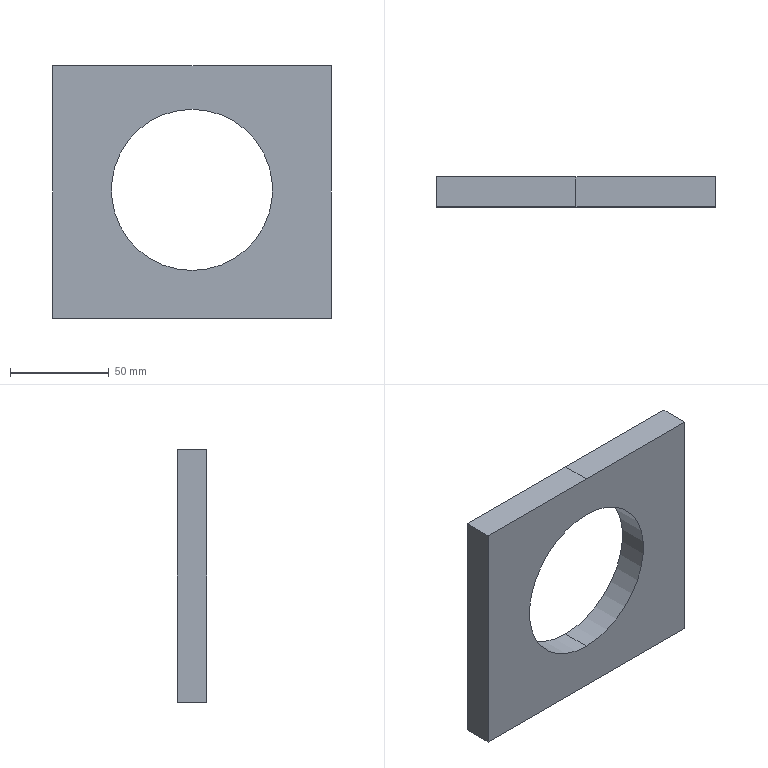Part | STEP file | 1 solid | 9 faces | box 140.887 x 15 x 127.87 mm | volume 191936 mm3 | plane 7 | cylinder 2 | commonest cylinder face diameters 81.521 x2
STEP:
#1=CARTESIAN_POINT('',(0.,0.,0.));
#2=DIRECTION('',(0.,0.,1.));
#3=DIRECTION('',(1.,0.,0.));
#4=AXIS2_PLACEMENT_3D('',#1,#2,#3);
#5=CARTESIAN_POINT('',(340.649,339.014,286.866));
#6=VERTEX_POINT('',#5);
#7=CARTESIAN_POINT('',(340.649,354.014,286.866));
#8=VERTEX_POINT('',#7);
#9=CARTESIAN_POINT('',(340.649,-550.01,286.866));
#10=DIRECTION('',(0.,1.,0.));
#11=VECTOR('',#10,1.);
#12=LINE('',#9,#11);
#13=CARTESIAN_POINT('',(340.649,-550.01,246.106));
#14=DIRECTION('',(0.,1.,0.));
#15=DIRECTION('',(0.,0.,1.));
#16=AXIS2_PLACEMENT_3D('',#13,#14,#15);
#17=CYLINDRICAL_SURFACE('',#16,40.761);
#18=CARTESIAN_POINT('',(6.283,0.));
#19=DIRECTION('',(0.,1.));
#20=VECTOR('',#19,1.);
#21=LINE('',#18,#20);
#22=(GEOMETRIC_REPRESENTATION_CONTEXT(2)PARAMETRIC_REPRESENTATION_CONTEXT()REPRESENTATION_CONTEXT('',''));
#23=DEFINITIONAL_REPRESENTATION('',(#21),#22);
#24=PCURVE('',#17,#23);
#25=CARTESIAN_POINT('',(340.649,-550.01,246.106));
#26=DIRECTION('',(0.,1.,0.));
#27=DIRECTION('',(0.,0.,1.));
#28=AXIS2_PLACEMENT_3D('',#25,#26,#27);
#29=CYLINDRICAL_SURFACE('',#28,40.761);
#30=CARTESIAN_POINT('',(0.,0.));
#31=DIRECTION('',(0.,1.));
#32=VECTOR('',#31,1.);
#33=LINE('',#30,#32);
#34=(GEOMETRIC_REPRESENTATION_CONTEXT(2)PARAMETRIC_REPRESENTATION_CONTEXT()REPRESENTATION_CONTEXT('',''));
#35=DEFINITIONAL_REPRESENTATION('',(#33),#34);
#36=PCURVE('',#29,#35);
#37=SURFACE_CURVE('',#12,(#24,#36),.PCURVE_S1.);
#38=EDGE_CURVE('',#6,#8,#37,.T.);
#39=ORIENTED_EDGE('',*,*,#38,.T.);
#40=CARTESIAN_POINT('',(340.649,354.014,205.345));
#41=VERTEX_POINT('',#40);
#42=CARTESIAN_POINT('',(340.649,354.014,246.106));
#43=DIRECTION('',(0.,1.,0.));
#44=DIRECTION('',(0.,0.,1.));
#45=AXIS2_PLACEMENT_3D('',#42,#43,#44);
#46=CIRCLE('',#45,40.761);
#47=CARTESIAN_POINT('',(0.,904.024));
#48=DIRECTION('',(1.,0.));
#49=VECTOR('',#48,1.);
#50=LINE('',#47,#49);
#51=(GEOMETRIC_REPRESENTATION_CONTEXT(2)PARAMETRIC_REPRESENTATION_CONTEXT()REPRESENTATION_CONTEXT('',''));
#52=DEFINITIONAL_REPRESENTATION('',(#50),#51);
#53=PCURVE('',#17,#52);
#54=CARTESIAN_POINT('',(0.,354.014,0.));
#55=DIRECTION('',(0.,1.,0.));
#56=DIRECTION('',(0.,0.,1.));
#57=AXIS2_PLACEMENT_3D('',#54,#55,#56);
#58=PLANE('',#57);
#59=CARTESIAN_POINT('',(246.106,340.649));
#60=DIRECTION('',(1.,0.));
#61=AXIS2_PLACEMENT_2D('',#59,#60);
#62=CIRCLE('',#61,40.761);
#63=(GEOMETRIC_REPRESENTATION_CONTEXT(2)PARAMETRIC_REPRESENTATION_CONTEXT()REPRESENTATION_CONTEXT('',''));
#64=DEFINITIONAL_REPRESENTATION('',(#62),#63);
#65=PCURVE('',#58,#64);
#66=SURFACE_CURVE('',#46,(#53,#65),.PCURVE_S1.);
#67=EDGE_CURVE('',#41,#8,#66,.T.);
#68=ORIENTED_EDGE('',*,*,#67,.F.);
#69=CARTESIAN_POINT('',(340.649,339.014,205.345));
#70=VERTEX_POINT('',#69);
#71=CARTESIAN_POINT('',(340.649,-550.01,205.345));
#72=DIRECTION('',(0.,1.,0.));
#73=VECTOR('',#72,1.);
#74=LINE('',#71,#73);
#75=CARTESIAN_POINT('',(3.142,0.));
#76=DIRECTION('',(0.,1.));
#77=VECTOR('',#76,1.);
#78=LINE('',#75,#77);
#79=(GEOMETRIC_REPRESENTATION_CONTEXT(2)PARAMETRIC_REPRESENTATION_CONTEXT()REPRESENTATION_CONTEXT('',''));
#80=DEFINITIONAL_REPRESENTATION('',(#78),#79);
#81=PCURVE('',#17,#80);
#82=CARTESIAN_POINT('',(3.142,0.));
#83=DIRECTION('',(0.,1.));
#84=VECTOR('',#83,1.);
#85=LINE('',#82,#84);
#86=(GEOMETRIC_REPRESENTATION_CONTEXT(2)PARAMETRIC_REPRESENTATION_CONTEXT()REPRESENTATION_CONTEXT('',''));
#87=DEFINITIONAL_REPRESENTATION('',(#85),#86);
#88=PCURVE('',#29,#87);
#89=SURFACE_CURVE('',#74,(#81,#88),.PCURVE_S1.);
#90=EDGE_CURVE('',#70,#41,#89,.T.);
#91=ORIENTED_EDGE('',*,*,#90,.F.);
#92=CARTESIAN_POINT('',(340.649,339.014,246.106));
#93=DIRECTION('',(0.,1.,0.));
#94=DIRECTION('',(0.,0.,1.));
#95=AXIS2_PLACEMENT_3D('',#92,#93,#94);
#96=CIRCLE('',#95,40.761);
#97=CARTESIAN_POINT('',(0.,889.024));
#98=DIRECTION('',(1.,0.));
#99=VECTOR('',#98,1.);
#100=LINE('',#97,#99);
#101=(GEOMETRIC_REPRESENTATION_CONTEXT(2)PARAMETRIC_REPRESENTATION_CONTEXT()REPRESENTATION_CONTEXT('',''));
#102=DEFINITIONAL_REPRESENTATION('',(#100),#101);
#103=PCURVE('',#17,#102);
#104=CARTESIAN_POINT('',(0.,339.014,0.));
#105=DIRECTION('',(0.,1.,0.));
#106=DIRECTION('',(0.,0.,1.));
#107=AXIS2_PLACEMENT_3D('',#104,#105,#106);
#108=PLANE('',#107);
#109=CARTESIAN_POINT('',(246.106,340.649));
#110=DIRECTION('',(1.,0.));
#111=AXIS2_PLACEMENT_2D('',#109,#110);
#112=CIRCLE('',#111,40.761);
#113=(GEOMETRIC_REPRESENTATION_CONTEXT(2)PARAMETRIC_REPRESENTATION_CONTEXT()REPRESENTATION_CONTEXT('',''));
#114=DEFINITIONAL_REPRESENTATION('',(#112),#113);
#115=PCURVE('',#108,#114);
#116=SURFACE_CURVE('',#96,(#103,#115),.PCURVE_S1.);
#117=EDGE_CURVE('',#70,#6,#116,.T.);
#118=ORIENTED_EDGE('',*,*,#117,.T.);
#119=EDGE_LOOP('',(#39,#68,#91,#118));
#120=FACE_BOUND('',#119,.F.);
#121=ADVANCED_FACE('',(#120),#17,.F.);
#122=CARTESIAN_POINT('',(340.649,354.014,246.106));
#123=DIRECTION('',(0.,1.,0.));
#124=DIRECTION('',(0.,0.,1.));
#125=AXIS2_PLACEMENT_3D('',#122,#123,#124);
#126=CIRCLE('',#125,40.761);
#127=CARTESIAN_POINT('',(0.,904.024));
#128=DIRECTION('',(1.,0.));
#129=VECTOR('',#128,1.);
#130=LINE('',#127,#129);
#131=(GEOMETRIC_REPRESENTATION_CONTEXT(2)PARAMETRIC_REPRESENTATION_CONTEXT()REPRESENTATION_CONTEXT('',''));
#132=DEFINITIONAL_REPRESENTATION('',(#130),#131);
#133=PCURVE('',#29,#132);
#134=CARTESIAN_POINT('',(246.106,340.649));
#135=DIRECTION('',(1.,0.));
#136=AXIS2_PLACEMENT_2D('',#134,#135);
#137=CIRCLE('',#136,40.761);
#138=(GEOMETRIC_REPRESENTATION_CONTEXT(2)PARAMETRIC_REPRESENTATION_CONTEXT()REPRESENTATION_CONTEXT('',''));
#139=DEFINITIONAL_REPRESENTATION('',(#137),#138);
#140=PCURVE('',#58,#139);
#141=SURFACE_CURVE('',#126,(#133,#140),.PCURVE_S1.);
#142=EDGE_CURVE('',#8,#41,#141,.T.);
#143=ORIENTED_EDGE('',*,*,#142,.F.);
#144=ORIENTED_EDGE('',*,*,#38,.F.);
#145=CARTESIAN_POINT('',(340.649,339.014,246.106));
#146=DIRECTION('',(0.,1.,0.));
#147=DIRECTION('',(0.,0.,1.));
#148=AXIS2_PLACEMENT_3D('',#145,#146,#147);
#149=CIRCLE('',#148,40.761);
#150=CARTESIAN_POINT('',(0.,889.024));
#151=DIRECTION('',(1.,0.));
#152=VECTOR('',#151,1.);
#153=LINE('',#150,#152);
#154=(GEOMETRIC_REPRESENTATION_CONTEXT(2)PARAMETRIC_REPRESENTATION_CONTEXT()REPRESENTATION_CONTEXT('',''));
#155=DEFINITIONAL_REPRESENTATION('',(#153),#154);
#156=PCURVE('',#29,#155);
#157=CARTESIAN_POINT('',(246.106,340.649));
#158=DIRECTION('',(1.,0.));
#159=AXIS2_PLACEMENT_2D('',#157,#158);
#160=CIRCLE('',#159,40.761);
#161=(GEOMETRIC_REPRESENTATION_CONTEXT(2)PARAMETRIC_REPRESENTATION_CONTEXT()REPRESENTATION_CONTEXT('',''));
#162=DEFINITIONAL_REPRESENTATION('',(#160),#161);
#163=PCURVE('',#108,#162);
#164=SURFACE_CURVE('',#149,(#156,#163),.PCURVE_S1.);
#165=EDGE_CURVE('',#6,#70,#164,.T.);
#166=ORIENTED_EDGE('',*,*,#165,.T.);
#167=ORIENTED_EDGE('',*,*,#90,.T.);
#168=EDGE_LOOP('',(#143,#144,#166,#167));
#169=FACE_BOUND('',#168,.F.);
#170=ADVANCED_FACE('',(#169),#29,.F.);
#171=ORIENTED_EDGE('',*,*,#165,.T.);
#172=ORIENTED_EDGE('',*,*,#117,.T.);
#173=EDGE_LOOP('',(#171,#172));
#174=FACE_BOUND('',#173,.T.);
#175=CARTESIAN_POINT('',(270.205,339.014,308.985));
#176=VERTEX_POINT('',#175);
#177=CARTESIAN_POINT('',(270.205,339.014,181.115));
#178=VERTEX_POINT('',#177);
#179=CARTESIAN_POINT('',(270.205,339.014,181.115));
#180=DIRECTION('',(0.,0.,-1.));
#181=VECTOR('',#180,1.);
#182=LINE('',#179,#181);
#183=CARTESIAN_POINT('',(181.115,270.205));
#184=DIRECTION('',(-1.,0.));
#185=VECTOR('',#184,1.);
#186=LINE('',#183,#185);
#187=(GEOMETRIC_REPRESENTATION_CONTEXT(2)PARAMETRIC_REPRESENTATION_CONTEXT()REPRESENTATION_CONTEXT('',''));
#188=DEFINITIONAL_REPRESENTATION('',(#186),#187);
#189=PCURVE('',#108,#188);
#190=CARTESIAN_POINT('',(270.205,339.014,181.115));
#191=DIRECTION('',(1.,0.,0.));
#192=DIRECTION('',(0.,0.,-1.));
#193=AXIS2_PLACEMENT_3D('',#190,#191,#192);
#194=PLANE('',#193);
#195=CARTESIAN_POINT('',(0.,0.));
#196=DIRECTION('',(1.,0.));
#197=VECTOR('',#196,1.);
#198=LINE('',#195,#197);
#199=(GEOMETRIC_REPRESENTATION_CONTEXT(2)PARAMETRIC_REPRESENTATION_CONTEXT()REPRESENTATION_CONTEXT('',''));
#200=DEFINITIONAL_REPRESENTATION('',(#198),#199);
#201=PCURVE('',#194,#200);
#202=SURFACE_CURVE('',#182,(#189,#201),.PCURVE_S1.);
#203=EDGE_CURVE('',#176,#178,#202,.T.);
#204=ORIENTED_EDGE('',*,*,#203,.T.);
#205=CARTESIAN_POINT('',(411.092,339.014,181.115));
#206=VERTEX_POINT('',#205);
#207=CARTESIAN_POINT('',(270.205,339.014,181.115));
#208=DIRECTION('',(1.,0.,0.));
#209=VECTOR('',#208,1.);
#210=LINE('',#207,#209);
#211=CARTESIAN_POINT('',(181.115,270.205));
#212=DIRECTION('',(0.,1.));
#213=VECTOR('',#212,1.);
#214=LINE('',#211,#213);
#215=(GEOMETRIC_REPRESENTATION_CONTEXT(2)PARAMETRIC_REPRESENTATION_CONTEXT()REPRESENTATION_CONTEXT('',''));
#216=DEFINITIONAL_REPRESENTATION('',(#214),#215);
#217=PCURVE('',#108,#216);
#218=CARTESIAN_POINT('',(270.205,339.014,181.115));
#219=DIRECTION('',(0.,0.,1.));
#220=DIRECTION('',(1.,0.,0.));
#221=AXIS2_PLACEMENT_3D('',#218,#219,#220);
#222=PLANE('',#221);
#223=CARTESIAN_POINT('',(0.,0.));
#224=DIRECTION('',(1.,0.));
#225=VECTOR('',#224,1.);
#226=LINE('',#223,#225);
#227=(GEOMETRIC_REPRESENTATION_CONTEXT(2)PARAMETRIC_REPRESENTATION_CONTEXT()REPRESENTATION_CONTEXT('',''));
#228=DEFINITIONAL_REPRESENTATION('',(#226),#227);
#229=PCURVE('',#222,#228);
#230=SURFACE_CURVE('',#210,(#217,#229),.PCURVE_S1.);
#231=EDGE_CURVE('',#178,#206,#230,.T.);
#232=ORIENTED_EDGE('',*,*,#231,.T.);
#233=CARTESIAN_POINT('',(411.092,339.014,308.985));
#234=VERTEX_POINT('',#233);
#235=CARTESIAN_POINT('',(411.092,339.014,181.115));
#236=DIRECTION('',(0.,0.,1.));
#237=VECTOR('',#236,1.);
#238=LINE('',#235,#237);
#239=CARTESIAN_POINT('',(181.115,411.092));
#240=DIRECTION('',(1.,0.));
#241=VECTOR('',#240,1.);
#242=LINE('',#239,#241);
#243=(GEOMETRIC_REPRESENTATION_CONTEXT(2)PARAMETRIC_REPRESENTATION_CONTEXT()REPRESENTATION_CONTEXT('',''));
#244=DEFINITIONAL_REPRESENTATION('',(#242),#243);
#245=PCURVE('',#108,#244);
#246=CARTESIAN_POINT('',(411.092,339.014,181.115));
#247=DIRECTION('',(-1.,0.,0.));
#248=DIRECTION('',(0.,0.,1.));
#249=AXIS2_PLACEMENT_3D('',#246,#247,#248);
#250=PLANE('',#249);
#251=CARTESIAN_POINT('',(0.,0.));
#252=DIRECTION('',(1.,0.));
#253=VECTOR('',#252,1.);
#254=LINE('',#251,#253);
#255=(GEOMETRIC_REPRESENTATION_CONTEXT(2)PARAMETRIC_REPRESENTATION_CONTEXT()REPRESENTATION_CONTEXT('',''));
#256=DEFINITIONAL_REPRESENTATION('',(#254),#255);
#257=PCURVE('',#250,#256);
#258=SURFACE_CURVE('',#238,(#245,#257),.PCURVE_S1.);
#259=EDGE_CURVE('',#206,#234,#258,.T.);
#260=ORIENTED_EDGE('',*,*,#259,.T.);
#261=CARTESIAN_POINT('',(340.649,339.014,308.985));
#262=VERTEX_POINT('',#261);
#263=CARTESIAN_POINT('',(270.205,339.014,308.985));
#264=DIRECTION('',(-1.,0.,0.));
#265=VECTOR('',#264,1.);
#266=LINE('',#263,#265);
#267=CARTESIAN_POINT('',(308.985,270.205));
#268=DIRECTION('',(0.,-1.));
#269=VECTOR('',#268,1.);
#270=LINE('',#267,#269);
#271=(GEOMETRIC_REPRESENTATION_CONTEXT(2)PARAMETRIC_REPRESENTATION_CONTEXT()REPRESENTATION_CONTEXT('',''));
#272=DEFINITIONAL_REPRESENTATION('',(#270),#271);
#273=PCURVE('',#108,#272);
#274=CARTESIAN_POINT('',(270.205,339.014,308.985));
#275=DIRECTION('',(0.,0.,-1.));
#276=DIRECTION('',(-1.,0.,0.));
#277=AXIS2_PLACEMENT_3D('',#274,#275,#276);
#278=PLANE('',#277);
#279=CARTESIAN_POINT('',(0.,0.));
#280=DIRECTION('',(1.,0.));
#281=VECTOR('',#280,1.);
#282=LINE('',#279,#281);
#283=(GEOMETRIC_REPRESENTATION_CONTEXT(2)PARAMETRIC_REPRESENTATION_CONTEXT()REPRESENTATION_CONTEXT('',''));
#284=DEFINITIONAL_REPRESENTATION('',(#282),#283);
#285=PCURVE('',#278,#284);
#286=SURFACE_CURVE('',#266,(#273,#285),.PCURVE_S1.);
#287=EDGE_CURVE('',#234,#262,#286,.T.);
#288=ORIENTED_EDGE('',*,*,#287,.T.);
#289=CARTESIAN_POINT('',(270.205,339.014,308.985));
#290=DIRECTION('',(-1.,0.,0.));
#291=VECTOR('',#290,1.);
#292=LINE('',#289,#291);
#293=CARTESIAN_POINT('',(308.985,270.205));
#294=DIRECTION('',(0.,-1.));
#295=VECTOR('',#294,1.);
#296=LINE('',#293,#295);
#297=(GEOMETRIC_REPRESENTATION_CONTEXT(2)PARAMETRIC_REPRESENTATION_CONTEXT()REPRESENTATION_CONTEXT('',''));
#298=DEFINITIONAL_REPRESENTATION('',(#296),#297);
#299=PCURVE('',#108,#298);
#300=CARTESIAN_POINT('',(270.205,339.014,308.985));
#301=DIRECTION('',(0.,0.,-1.));
#302=DIRECTION('',(-1.,0.,0.));
#303=AXIS2_PLACEMENT_3D('',#300,#301,#302);
#304=PLANE('',#303);
#305=CARTESIAN_POINT('',(0.,0.));
#306=DIRECTION('',(1.,0.));
#307=VECTOR('',#306,1.);
#308=LINE('',#305,#307);
#309=(GEOMETRIC_REPRESENTATION_CONTEXT(2)PARAMETRIC_REPRESENTATION_CONTEXT()REPRESENTATION_CONTEXT('',''));
#310=DEFINITIONAL_REPRESENTATION('',(#308),#309);
#311=PCURVE('',#304,#310);
#312=SURFACE_CURVE('',#292,(#299,#311),.PCURVE_S1.);
#313=EDGE_CURVE('',#262,#176,#312,.T.);
#314=ORIENTED_EDGE('',*,*,#313,.T.);
#315=EDGE_LOOP('',(#204,#232,#260,#288,#314));
#316=FACE_BOUND('',#315,.T.);
#317=ADVANCED_FACE('',(#174,#316),#108,.F.);
#318=ORIENTED_EDGE('',*,*,#142,.F.);
#319=ORIENTED_EDGE('',*,*,#67,.F.);
#320=EDGE_LOOP('',(#318,#319));
#321=FACE_BOUND('',#320,.T.);
#322=CARTESIAN_POINT('',(270.205,354.014,308.985));
#323=VERTEX_POINT('',#322);
#324=CARTESIAN_POINT('',(270.205,354.014,181.115));
#325=VERTEX_POINT('',#324);
#326=CARTESIAN_POINT('',(270.205,354.014,181.115));
#327=DIRECTION('',(0.,0.,-1.));
#328=VECTOR('',#327,1.);
#329=LINE('',#326,#328);
#330=CARTESIAN_POINT('',(181.115,270.205));
#331=DIRECTION('',(-1.,0.));
#332=VECTOR('',#331,1.);
#333=LINE('',#330,#332);
#334=(GEOMETRIC_REPRESENTATION_CONTEXT(2)PARAMETRIC_REPRESENTATION_CONTEXT()REPRESENTATION_CONTEXT('',''));
#335=DEFINITIONAL_REPRESENTATION('',(#333),#334);
#336=PCURVE('',#58,#335);
#337=CARTESIAN_POINT('',(0.,15.));
#338=DIRECTION('',(1.,0.));
#339=VECTOR('',#338,1.);
#340=LINE('',#337,#339);
#341=(GEOMETRIC_REPRESENTATION_CONTEXT(2)PARAMETRIC_REPRESENTATION_CONTEXT()REPRESENTATION_CONTEXT('',''));
#342=DEFINITIONAL_REPRESENTATION('',(#340),#341);
#343=PCURVE('',#194,#342);
#344=SURFACE_CURVE('',#329,(#336,#343),.PCURVE_S1.);
#345=EDGE_CURVE('',#323,#325,#344,.T.);
#346=ORIENTED_EDGE('',*,*,#345,.F.);
#347=CARTESIAN_POINT('',(340.649,354.014,308.985));
#348=VERTEX_POINT('',#347);
#349=CARTESIAN_POINT('',(270.205,354.014,308.985));
#350=DIRECTION('',(-1.,0.,0.));
#351=VECTOR('',#350,1.);
#352=LINE('',#349,#351);
#353=CARTESIAN_POINT('',(308.985,270.205));
#354=DIRECTION('',(0.,-1.));
#355=VECTOR('',#354,1.);
#356=LINE('',#353,#355);
#357=(GEOMETRIC_REPRESENTATION_CONTEXT(2)PARAMETRIC_REPRESENTATION_CONTEXT()REPRESENTATION_CONTEXT('',''));
#358=DEFINITIONAL_REPRESENTATION('',(#356),#357);
#359=PCURVE('',#58,#358);
#360=CARTESIAN_POINT('',(0.,15.));
#361=DIRECTION('',(1.,0.));
#362=VECTOR('',#361,1.);
#363=LINE('',#360,#362);
#364=(GEOMETRIC_REPRESENTATION_CONTEXT(2)PARAMETRIC_REPRESENTATION_CONTEXT()REPRESENTATION_CONTEXT('',''));
#365=DEFINITIONAL_REPRESENTATION('',(#363),#364);
#366=PCURVE('',#304,#365);
#367=SURFACE_CURVE('',#352,(#359,#366),.PCURVE_S1.);
#368=EDGE_CURVE('',#348,#323,#367,.T.);
#369=ORIENTED_EDGE('',*,*,#368,.F.);
#370=CARTESIAN_POINT('',(411.092,354.014,308.985));
#371=VERTEX_POINT('',#370);
#372=CARTESIAN_POINT('',(270.205,354.014,308.985));
#373=DIRECTION('',(-1.,0.,0.));
#374=VECTOR('',#373,1.);
#375=LINE('',#372,#374);
#376=CARTESIAN_POINT('',(308.985,270.205));
#377=DIRECTION('',(0.,-1.));
#378=VECTOR('',#377,1.);
#379=LINE('',#376,#378);
#380=(GEOMETRIC_REPRESENTATION_CONTEXT(2)PARAMETRIC_REPRESENTATION_CONTEXT()REPRESENTATION_CONTEXT('',''));
#381=DEFINITIONAL_REPRESENTATION('',(#379),#380);
#382=PCURVE('',#58,#381);
#383=CARTESIAN_POINT('',(0.,15.));
#384=DIRECTION('',(1.,0.));
#385=VECTOR('',#384,1.);
#386=LINE('',#383,#385);
#387=(GEOMETRIC_REPRESENTATION_CONTEXT(2)PARAMETRIC_REPRESENTATION_CONTEXT()REPRESENTATION_CONTEXT('',''));
#388=DEFINITIONAL_REPRESENTATION('',(#386),#387);
#389=PCURVE('',#278,#388);
#390=SURFACE_CURVE('',#375,(#382,#389),.PCURVE_S1.);
#391=EDGE_CURVE('',#371,#348,#390,.T.);
#392=ORIENTED_EDGE('',*,*,#391,.F.);
#393=CARTESIAN_POINT('',(411.092,354.014,181.115));
#394=VERTEX_POINT('',#393);
#395=CARTESIAN_POINT('',(411.092,354.014,181.115));
#396=DIRECTION('',(0.,0.,1.));
#397=VECTOR('',#396,1.);
#398=LINE('',#395,#397);
#399=CARTESIAN_POINT('',(181.115,411.092));
#400=DIRECTION('',(1.,0.));
#401=VECTOR('',#400,1.);
#402=LINE('',#399,#401);
#403=(GEOMETRIC_REPRESENTATION_CONTEXT(2)PARAMETRIC_REPRESENTATION_CONTEXT()REPRESENTATION_CONTEXT('',''));
#404=DEFINITIONAL_REPRESENTATION('',(#402),#403);
#405=PCURVE('',#58,#404);
#406=CARTESIAN_POINT('',(0.,15.));
#407=DIRECTION('',(1.,0.));
#408=VECTOR('',#407,1.);
#409=LINE('',#406,#408);
#410=(GEOMETRIC_REPRESENTATION_CONTEXT(2)PARAMETRIC_REPRESENTATION_CONTEXT()REPRESENTATION_CONTEXT('',''));
#411=DEFINITIONAL_REPRESENTATION('',(#409),#410);
#412=PCURVE('',#250,#411);
#413=SURFACE_CURVE('',#398,(#405,#412),.PCURVE_S1.);
#414=EDGE_CURVE('',#394,#371,#413,.T.);
#415=ORIENTED_EDGE('',*,*,#414,.F.);
#416=CARTESIAN_POINT('',(270.205,354.014,181.115));
#417=DIRECTION('',(1.,0.,0.));
#418=VECTOR('',#417,1.);
#419=LINE('',#416,#418);
#420=CARTESIAN_POINT('',(181.115,270.205));
#421=DIRECTION('',(0.,1.));
#422=VECTOR('',#421,1.);
#423=LINE('',#420,#422);
#424=(GEOMETRIC_REPRESENTATION_CONTEXT(2)PARAMETRIC_REPRESENTATION_CONTEXT()REPRESENTATION_CONTEXT('',''));
#425=DEFINITIONAL_REPRESENTATION('',(#423),#424);
#426=PCURVE('',#58,#425);
#427=CARTESIAN_POINT('',(0.,15.));
#428=DIRECTION('',(1.,0.));
#429=VECTOR('',#428,1.);
#430=LINE('',#427,#429);
#431=(GEOMETRIC_REPRESENTATION_CONTEXT(2)PARAMETRIC_REPRESENTATION_CONTEXT()REPRESENTATION_CONTEXT('',''));
#432=DEFINITIONAL_REPRESENTATION('',(#430),#431);
#433=PCURVE('',#222,#432);
#434=SURFACE_CURVE('',#419,(#426,#433),.PCURVE_S1.);
#435=EDGE_CURVE('',#325,#394,#434,.T.);
#436=ORIENTED_EDGE('',*,*,#435,.F.);
#437=EDGE_LOOP('',(#346,#369,#392,#415,#436));
#438=FACE_BOUND('',#437,.T.);
#439=ADVANCED_FACE('',(#321,#438),#58,.T.);
#440=ORIENTED_EDGE('',*,*,#345,.T.);
#441=CARTESIAN_POINT('',(270.205,339.014,181.115));
#442=DIRECTION('',(0.,1.,0.));
#443=VECTOR('',#442,1.);
#444=LINE('',#441,#443);
#445=CARTESIAN_POINT('',(0.,0.));
#446=DIRECTION('',(0.,1.));
#447=VECTOR('',#446,1.);
#448=LINE('',#445,#447);
#449=(GEOMETRIC_REPRESENTATION_CONTEXT(2)PARAMETRIC_REPRESENTATION_CONTEXT()REPRESENTATION_CONTEXT('',''));
#450=DEFINITIONAL_REPRESENTATION('',(#448),#449);
#451=PCURVE('',#194,#450);
#452=CARTESIAN_POINT('',(0.,0.));
#453=DIRECTION('',(0.,1.));
#454=VECTOR('',#453,1.);
#455=LINE('',#452,#454);
#456=(GEOMETRIC_REPRESENTATION_CONTEXT(2)PARAMETRIC_REPRESENTATION_CONTEXT()REPRESENTATION_CONTEXT('',''));
#457=DEFINITIONAL_REPRESENTATION('',(#455),#456);
#458=PCURVE('',#222,#457);
#459=SURFACE_CURVE('',#444,(#451,#458),.PCURVE_S1.);
#460=EDGE_CURVE('',#178,#325,#459,.T.);
#461=ORIENTED_EDGE('',*,*,#460,.F.);
#462=ORIENTED_EDGE('',*,*,#203,.F.);
#463=CARTESIAN_POINT('',(270.205,339.014,308.985));
#464=DIRECTION('',(0.,1.,0.));
#465=VECTOR('',#464,1.);
#466=LINE('',#463,#465);
#467=CARTESIAN_POINT('',(-127.87,0.));
#468=DIRECTION('',(0.,1.));
#469=VECTOR('',#468,1.);
#470=LINE('',#467,#469);
#471=(GEOMETRIC_REPRESENTATION_CONTEXT(2)PARAMETRIC_REPRESENTATION_CONTEXT()REPRESENTATION_CONTEXT('',''));
#472=DEFINITIONAL_REPRESENTATION('',(#470),#471);
#473=PCURVE('',#194,#472);
#474=CARTESIAN_POINT('',(0.,0.));
#475=DIRECTION('',(0.,1.));
#476=VECTOR('',#475,1.);
#477=LINE('',#474,#476);
#478=(GEOMETRIC_REPRESENTATION_CONTEXT(2)PARAMETRIC_REPRESENTATION_CONTEXT()REPRESENTATION_CONTEXT('',''));
#479=DEFINITIONAL_REPRESENTATION('',(#477),#478);
#480=PCURVE('',#304,#479);
#481=SURFACE_CURVE('',#466,(#473,#480),.PCURVE_S1.);
#482=EDGE_CURVE('',#176,#323,#481,.T.);
#483=ORIENTED_EDGE('',*,*,#482,.T.);
#484=EDGE_LOOP('',(#440,#461,#462,#483));
#485=FACE_BOUND('',#484,.T.);
#486=ADVANCED_FACE('',(#485),#194,.F.);
#487=CARTESIAN_POINT('',(340.649,339.014,308.985));
#488=DIRECTION('',(0.,-1.,0.));
#489=VECTOR('',#488,1.);
#490=LINE('',#487,#489);
#491=CARTESIAN_POINT('',(-70.444,0.));
#492=DIRECTION('',(0.,-1.));
#493=VECTOR('',#492,1.);
#494=LINE('',#491,#493);
#495=(GEOMETRIC_REPRESENTATION_CONTEXT(2)PARAMETRIC_REPRESENTATION_CONTEXT()REPRESENTATION_CONTEXT('',''));
#496=DEFINITIONAL_REPRESENTATION('',(#494),#495);
#497=PCURVE('',#304,#496);
#498=CARTESIAN_POINT('',(-70.444,0.));
#499=DIRECTION('',(0.,-1.));
#500=VECTOR('',#499,1.);
#501=LINE('',#498,#500);
#502=(GEOMETRIC_REPRESENTATION_CONTEXT(2)PARAMETRIC_REPRESENTATION_CONTEXT()REPRESENTATION_CONTEXT('',''));
#503=DEFINITIONAL_REPRESENTATION('',(#501),#502);
#504=PCURVE('',#278,#503);
#505=SURFACE_CURVE('',#490,(#497,#504),.PCURVE_S1.);
#506=EDGE_CURVE('',#348,#262,#505,.T.);
#507=ORIENTED_EDGE('',*,*,#506,.F.);
#508=ORIENTED_EDGE('',*,*,#368,.T.);
#509=ORIENTED_EDGE('',*,*,#482,.F.);
#510=ORIENTED_EDGE('',*,*,#313,.F.);
#511=EDGE_LOOP('',(#507,#508,#509,#510));
#512=FACE_BOUND('',#511,.T.);
#513=ADVANCED_FACE('',(#512),#304,.F.);
#514=ORIENTED_EDGE('',*,*,#391,.T.);
#515=ORIENTED_EDGE('',*,*,#506,.T.);
#516=ORIENTED_EDGE('',*,*,#287,.F.);
#517=CARTESIAN_POINT('',(411.092,339.014,308.985));
#518=DIRECTION('',(0.,1.,0.));
#519=VECTOR('',#518,1.);
#520=LINE('',#517,#519);
#521=CARTESIAN_POINT('',(-140.887,0.));
#522=DIRECTION('',(0.,1.));
#523=VECTOR('',#522,1.);
#524=LINE('',#521,#523);
#525=(GEOMETRIC_REPRESENTATION_CONTEXT(2)PARAMETRIC_REPRESENTATION_CONTEXT()REPRESENTATION_CONTEXT('',''));
#526=DEFINITIONAL_REPRESENTATION('',(#524),#525);
#527=PCURVE('',#278,#526);
#528=CARTESIAN_POINT('',(127.87,0.));
#529=DIRECTION('',(0.,1.));
#530=VECTOR('',#529,1.);
#531=LINE('',#528,#530);
#532=(GEOMETRIC_REPRESENTATION_CONTEXT(2)PARAMETRIC_REPRESENTATION_CONTEXT()REPRESENTATION_CONTEXT('',''));
#533=DEFINITIONAL_REPRESENTATION('',(#531),#532);
#534=PCURVE('',#250,#533);
#535=SURFACE_CURVE('',#520,(#527,#534),.PCURVE_S1.);
#536=EDGE_CURVE('',#234,#371,#535,.T.);
#537=ORIENTED_EDGE('',*,*,#536,.T.);
#538=EDGE_LOOP('',(#514,#515,#516,#537));
#539=FACE_BOUND('',#538,.T.);
#540=ADVANCED_FACE('',(#539),#278,.F.);
#541=ORIENTED_EDGE('',*,*,#414,.T.);
#542=ORIENTED_EDGE('',*,*,#536,.F.);
#543=ORIENTED_EDGE('',*,*,#259,.F.);
#544=CARTESIAN_POINT('',(411.092,339.014,181.115));
#545=DIRECTION('',(0.,1.,0.));
#546=VECTOR('',#545,1.);
#547=LINE('',#544,#546);
#548=CARTESIAN_POINT('',(0.,0.));
#549=DIRECTION('',(0.,1.));
#550=VECTOR('',#549,1.);
#551=LINE('',#548,#550);
#552=(GEOMETRIC_REPRESENTATION_CONTEXT(2)PARAMETRIC_REPRESENTATION_CONTEXT()REPRESENTATION_CONTEXT('',''));
#553=DEFINITIONAL_REPRESENTATION('',(#551),#552);
#554=PCURVE('',#250,#553);
#555=CARTESIAN_POINT('',(140.887,0.));
#556=DIRECTION('',(0.,1.));
#557=VECTOR('',#556,1.);
#558=LINE('',#555,#557);
#559=(GEOMETRIC_REPRESENTATION_CONTEXT(2)PARAMETRIC_REPRESENTATION_CONTEXT()REPRESENTATION_CONTEXT('',''));
#560=DEFINITIONAL_REPRESENTATION('',(#558),#559);
#561=PCURVE('',#222,#560);
#562=SURFACE_CURVE('',#547,(#554,#561),.PCURVE_S1.);
#563=EDGE_CURVE('',#206,#394,#562,.T.);
#564=ORIENTED_EDGE('',*,*,#563,.T.);
#565=EDGE_LOOP('',(#541,#542,#543,#564));
#566=FACE_BOUND('',#565,.T.);
#567=ADVANCED_FACE('',(#566),#250,.F.);
#568=ORIENTED_EDGE('',*,*,#435,.T.);
#569=ORIENTED_EDGE('',*,*,#563,.F.);
#570=ORIENTED_EDGE('',*,*,#231,.F.);
#571=ORIENTED_EDGE('',*,*,#460,.T.);
#572=EDGE_LOOP('',(#568,#569,#570,#571));
#573=FACE_BOUND('',#572,.T.);
#574=ADVANCED_FACE('',(#573),#222,.F.);
#575=CLOSED_SHELL('',(#121,#170,#317,#439,#486,#513,#540,#567,#574));
#576=MANIFOLD_SOLID_BREP('',#575);
#577=(LENGTH_UNIT()NAMED_UNIT(*)SI_UNIT(.MILLI.,.METRE.));
#578=UNCERTAINTY_MEASURE_WITH_UNIT(LENGTH_MEASURE(0.0000001),#577,'','');
#579=(NAMED_UNIT(*)PLANE_ANGLE_UNIT()SI_UNIT($,.RADIAN.));
#580=(NAMED_UNIT(*)SI_UNIT($,.STERADIAN.)SOLID_ANGLE_UNIT());
#581=(GEOMETRIC_REPRESENTATION_CONTEXT(3)GLOBAL_UNCERTAINTY_ASSIGNED_CONTEXT((#578))GLOBAL_UNIT_ASSIGNED_CONTEXT((#577,#579,#580))REPRESENTATION_CONTEXT('',''));
#582=ADVANCED_BREP_SHAPE_REPRESENTATION('',(#4,#576),#581);